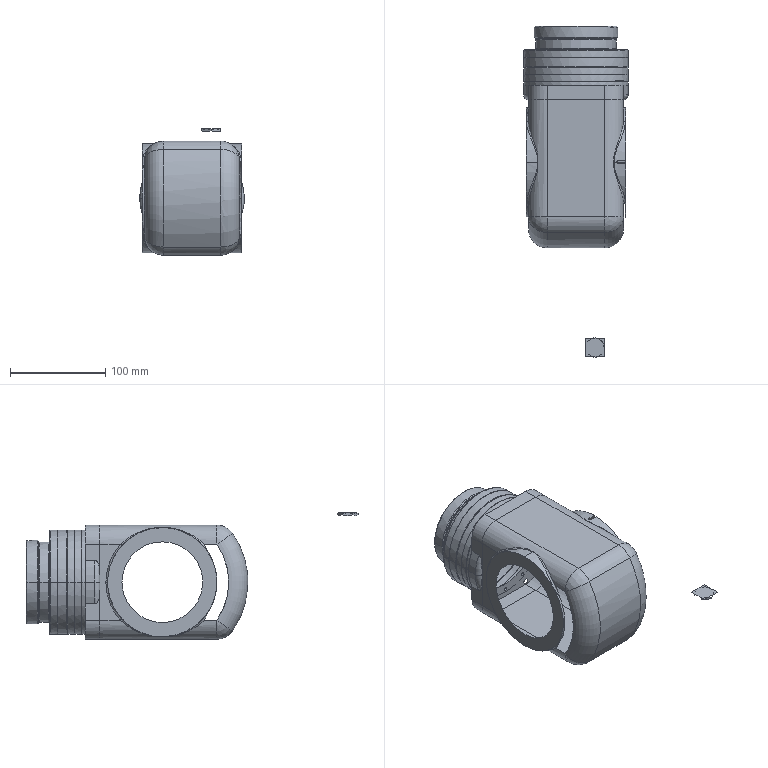Part | NX | features BREP 8 | 1 solid | 188 faces | box 110 x 349.47 x 133 mm | volume 1961121 mm3 | cylinder 104 | plane 30 | cone 27 | torus 18 | spline 5 | sphere 4 | commonest cylinder face diameters 8 x32 5 x16 4.5 x14 40 x10 110 x7 109.8 x6